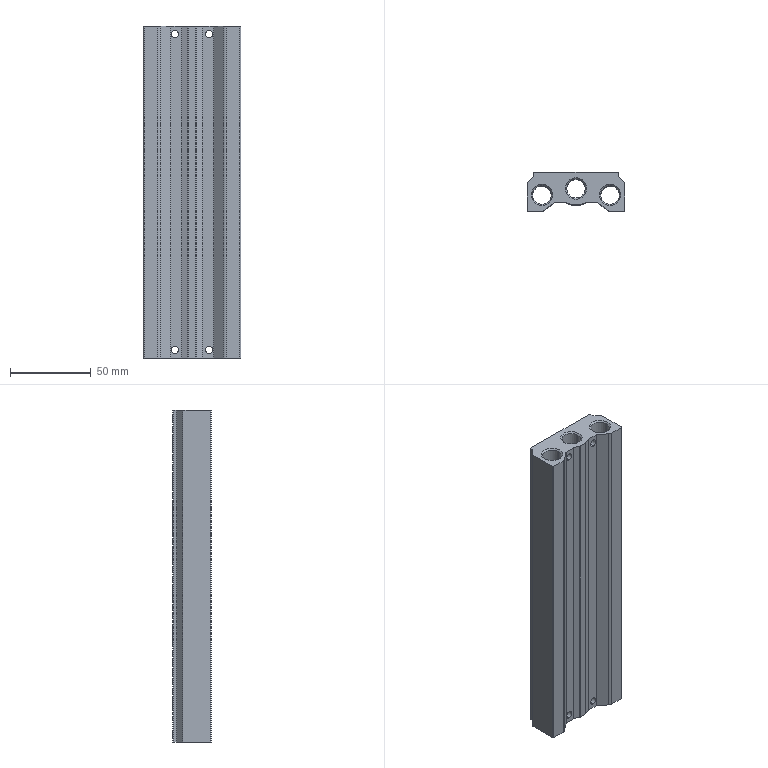Part | SolidWorks | features BaseBody 1 | 1 solid | 218 faces | box 60 x 24 x 205 mm | volume 179716 mm3 | cylinder 108 | cone 76 | plane 34 | commonest cylinder face diameters 2.459 x32 6.5 x32 10.2 x16 1 x12 4.5 x8 11.445 x6